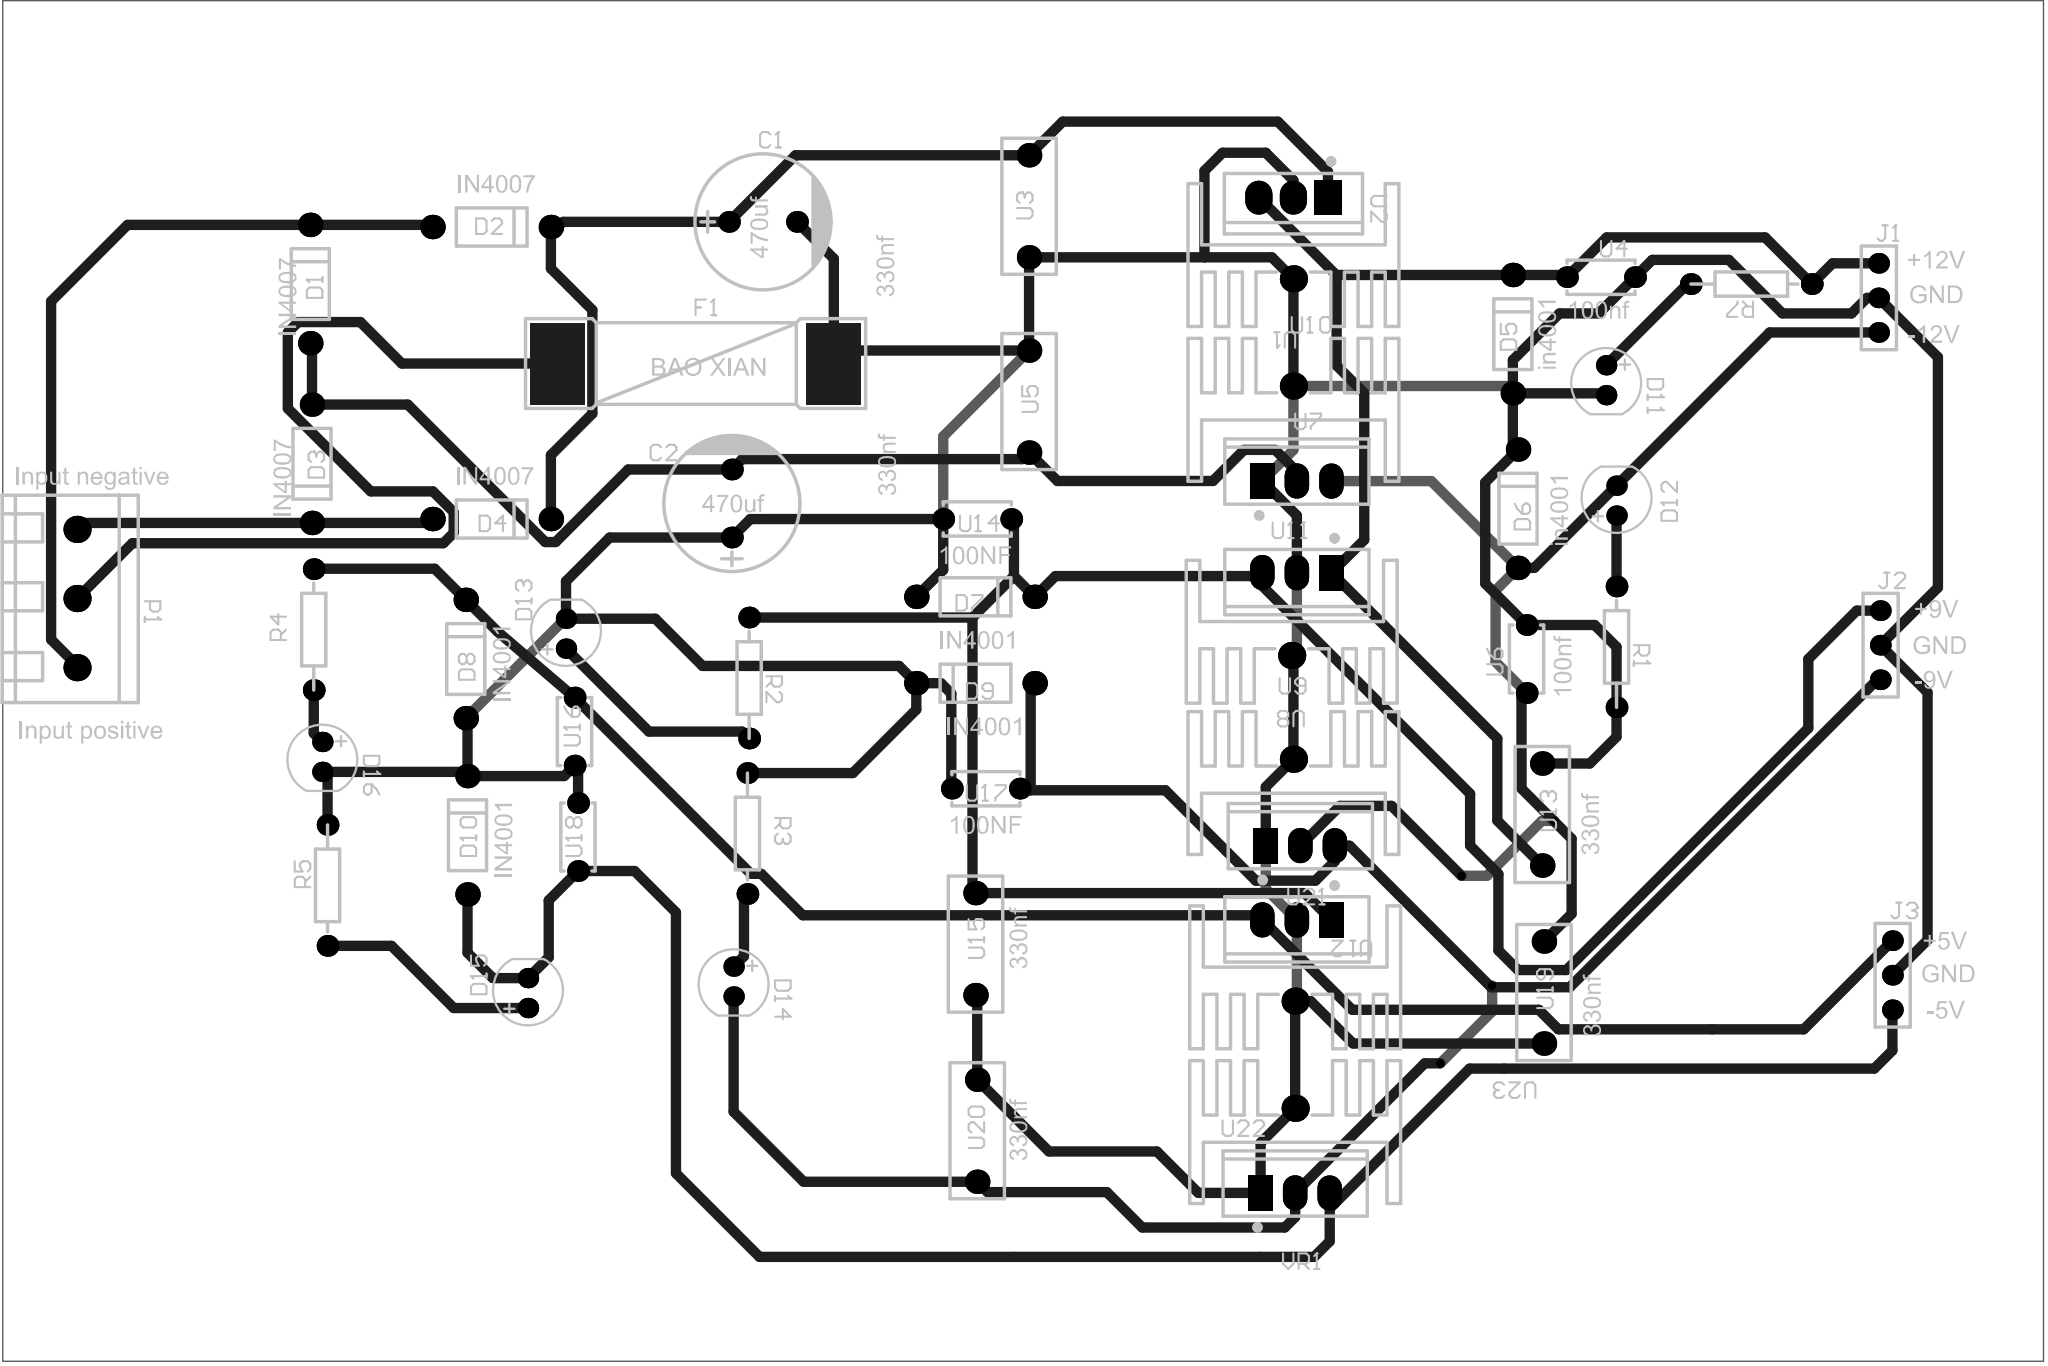Circuit board layout | Altium Designer
Layer stack:
# Altium Designer layer stack of  (unit mm; dielectric type: 0 none, 1 core, 2 prepreg, 3 surface material)
index,name,kind,layer,copper_thickness_mm,dielectric_type,dielectric_thickness_mm,dielectric_material,dielectric_constant
0,Top Silkscreen Layer,other,,,,,,
1,Top Paste Mask Layer,other,,,,,,
2,Top Solder Mask Layer,dielectric,,,3,0,,0
3,Top Layer,copper,Top Layer,0,,,,
4,Substrate-1,dielectric,,,3,0,,0
5,Bottom Layer,copper,Bottom Layer,0,,,,
6,Bottom Solder Mask Layer,dielectric,,,3,0,,0
7,Bottom Paste Mask Layer,other,,,,,,
8,Bottom Silkscreen Layer,other,,,,,,
# drill layer pairs: low layer,high layer
drill_pair,Top Layer,Bottom Layer
Part placement:
Designator,Comment,Layer,Footprint,Center-X(mm),Center-Y(mm),Rotation
D16,Red,TopLayer,发光二极管,99.794,120.617,270
D15,Red,TopLayer,发光二极管,114.907,103.259,90
D14,Red,TopLayer,发光二极管,130.02,104.107,270
D13,Red,TopLayer,发光二极管,117.701,129.675,90
D12,Red,TopLayer,发光二极管,194.917,139.454,90
D11,Red,TopLayer,发光二极管,194.155,148.303,270
VR1,L7905,TopLayer,TO-220-3_L10.0-W4.5-P2.54-L,171.295,88.57,0
U21,LM7909CT,TopLayer,TO-220-3_L10.0-W4.5-P2.54-L,171.676,114.097,0
U12,L7805CV-DG,TopLayer,TO-220-3_L10.0-W4.5-P2.54-L,171.422,108.636,180
U11,L7809CV,TopLayer,TO-220-3_L10.0-W4.5-P2.54-L,171.422,134.163,180
U7,L7912CV,TopLayer,TO-220-3_L10.0-W4.5-P2.54-L,171.422,140.894,0
U18,100NF,TopLayer,CAP-TH_L5.0-W2.5-P5.00-D1.0,118.59,114.732,270
U17,100NF,TopLayer,CAP-TH_L5.0-W2.5-P5.00-D1.0,148.562,118.288,0
U16,100NF,TopLayer,CAP-TH_L5.0-W2.5-P5.00-D1.0,118.336,122.479,270
U14,100NF,TopLayer,CAP-TH_L5.0-W2.5-P5.00-D1.0,147.927,138.1,180
U6,100NF,TopLayer,CAP-TH_L5.0-W2.5-P5.00-D1.0,188.313,127.813,270
U4,100NF,TopLayer,CAP-TH_L5.0-W2.5-P5.00-D1.0,193.774,155.88,0
U20,330nF,TopLayer,CAP-TH_L10.0-W4.0-P7.50-D0.6-1,147.927,93.142,90
U19,330nF,TopLayer,CAP-TH_L10.0-W4.0-P7.50-D0.6-1,189.583,103.302,270
U15,330nF,TopLayer,CAP-TH_L10.0-W4.0-P7.50-D0.6-1,147.8,106.858,90
U13,330nF,TopLayer,CAP-TH_L10.0-W4.0-P7.50-D0.6-1,189.456,116.383,270
U5,330nF,TopLayer,CAP-TH_L10.0-W4.0-P7.50-D0.6-1,151.737,146.736,90
U3,330nF,TopLayer,CAP-TH_L10.0-W4.0-P7.50-D0.6-1,151.737,161.087,90
U2,L7812CV,TopLayer,TO-220-3_L10.0-W4.5-P2.54-T,171.168,161.722,270
U23,15*10.5*21,TopLayer,SINK-TH_L15.0-W10.5-H21.0,171.295,102.667,180
U22,15*10.5*21,TopLayer,SINK-TH_L15.0-W10.5-H21.0,171.295,94.793,0
U10,15*10.5*21,TopLayer,SINK-TH_L15.0-W10.5-H21.0,171.168,147.879,0
U9,15*10.5*21,TopLayer,SINK-TH_L15.0-W10.5-H21.0,171.168,120.447,0
U8,15*10.5*21,TopLayer,SINK-TH_L15.0-W10.5-H21.0,171.041,128.067,180
U1,15*10.5*21,TopLayer,SINK-TH_L15.0-W10.5-H21.0,171.168,155.753,180
R7,10k 1/4W,TopLayer,10KÖ±²åµç×è_PCB·â×°,204.823,155.372,180
R5,10k 1/4W,TopLayer,10KÖ±²åµç×è_PCB·â×°,100.175,111.176,90
R4,10k 1/4W,TopLayer,10KÖ±²åµç×è_PCB·â×°,99.159,129.972,270
R3,10k 1/4W,TopLayer,10KÖ±²åµç×è_PCB·â×°,131.036,114.986,90
R2,10k 1/4W,TopLayer,10KÖ±²åµç×è_PCB·â×°,131.163,126.416,270
R1,10k 1/4W,TopLayer,10KÖ±²åµç×è_PCB·â×°,194.917,128.702,270
P1,WJ500V-5.08-3P,TopLayer,CONN-TH_3P-P5.00_WJ500V-5.08-3P,81.76,132.258,270
J3,1*3 pin header,TopLayer,1*3排针,215.194,104.572,0
J2,1*3 pin header,TopLayer,1*3排针,214.305,128.829,0
J1,1*3 pin header,TopLayer,1*3排针,214.178,154.356,0
F1,10A,TopLayer,FUSE-SMD_5-20MM,127.226,149.53,0
D10,IN4001,TopLayer,DO-41_BD2.4-L4.7-P8.70-D0.9-RD,110.462,114.859,270
D9,IN4001,TopLayer,DO-41_BD2.4-L4.7-P8.70-D0.9-RD,147.8,126.035,0
D8,IN4001,TopLayer,DO-41_BD2.4-L4.7-P8.70-D0.9-RD,110.335,127.813,270
D7,IN4001,TopLayer,DO-41_BD2.4-L4.7-P8.70-D0.9-RD,147.8,132.385,180
D6,IN4001,TopLayer,DO-41_BD2.4-L4.7-P8.70-D0.9-RD,187.678,138.862,270
D5,IN4001,TopLayer,DO-41_BD2.4-L4.7-P8.70-D0.9-RD,187.297,151.689,270
D4,1N4007,TopLayer,DO-41_BD2.4-L4.7-P8.70-D0.9-RD,112.24,138.1,180
D3,1N4007,TopLayer,DO-41_BD2.4-L4.7-P8.70-D0.9-RD,99.032,142.164,90
D2,1N4007,TopLayer,DO-41_BD2.4-L4.7-P8.70-D0.9-RD,112.24,159.563,180
D1,1N4007,TopLayer,DO-41_BD2.4-L4.7-P8.70-D0.9-RD,98.905,155.372,270
C2,470uF,TopLayer,CAP-TH_BD10.0-P5.00-D0.6-FD,129.893,139.243,90
C1,470uF,TopLayer,CAP-TH_BD10.0-P5.00-D0.6-FD,132.179,159.944,0
Pad and via stacks:
# Altium Designer via and pad stacks of  (unit mm). Each distinct definition once, with the count of objects using it.
# via: kind,start_layer,end_layer,hole_mm,diameter_mm,mode(0 simple;1 top-mid-bottom;2 full stack),diameter_per_layer,count,example_net
# pad: kind,layer,hole_mm,hole_type(0 round;1 square;2 slot),plating,top_size,top_shape(1 round;2 rect;3 octagon;9 rounded rect),mid_size,bottom_size,mode,footprint,size_per_layer,count,example
pad,Multi-Layer,0.8001,2,plated,1.5x1.5,1,1.5x1.5,1.5x1.5,0,\u00B7\u00A2\u00B9\u00E2\u00B6\u00FE\u00BC\u00AB\u00B9\u00DC,,12,D16.1
pad,Multi-Layer,1.2,2,plated,1.8x2.6,1,1.8x2.6,1.8x2.6,0,TO-220-3_L10.0-W4.5-P2.54-L,,2,VR1.2
pad,Multi-Layer,1.2,2,plated,1.8x2.6,2,1.8x2.6,1.8x2.6,0,TO-220-3_L10.0-W4.5-P2.54-L,,1,VR1.1
pad,Multi-Layer,1.2,0,plated,1.8x2.6,1,1.8x2.6,1.8x2.6,0,TO-220-3_L10.0-W4.5-P2.54-L,,8,U21.2
pad,Multi-Layer,1.2,0,plated,1.8x2.6,2,1.8x2.6,1.8x2.6,0,TO-220-3_L10.0-W4.5-P2.54-L,,4,U21.1
pad,Multi-Layer,1,0,plated,1.6x1.6,1,1.6x1.6,1.6x1.6,0,CAP-TH_L5.0-W2.5-P5.00-D1.0,,12,U18.1
pad,Multi-Layer,1,0,plated,1.8x1.8,1,1.8x1.8,1.8x1.8,0,CAP-TH_L10.0-W4.0-P7.50-D0.6-1,,12,U20.2
pad,Multi-Layer,1.3,0,plated,2x2.5,2,2x2.5,2x2.5,0,TO-220-3_L10.0-W4.5-P2.54-T,,1,U2.1
pad,Multi-Layer,1.3,0,plated,2x2.5,1,2x2.5,2x2.5,0,TO-220-3_L10.0-W4.5-P2.54-T,,2,U2.3
pad,Multi-Layer,1.5,0,plated,2x2,1,2x2,2x2,0,SINK-TH_L15.0-W10.5-H21.0,,6,U23.1
pad,Multi-Layer,0.92,2,plated,1.6x1.6,1,1.6x1.6,1.6x1.6,0,10K\u00D6\u00B1\u00B2\u00E5\u00B5\u00E7\u00D7\u00E8 PCB\u00B7\u00E2\u00D7\u00B0,,12,R7.1
pad,Multi-Layer,1.3,0,plated,2x2,1,2x2,2x2,0,CONN-TH_3P-P5.00_WJ500V-5.08-3P,,3,P1.3
pad,Multi-Layer,0.9144,0,plated,1.524x1.524,1,1.524x1.524,1.524x1.524,0,1*3\u00C5\u00C5\u00D5\u00EB,,9,J3.3
pad,Multi-Layer,1,0,plated,1.8x1.8,1,1.8x1.8,1.8x1.8,0,DO-41_BD2.4-L4.7-P8.70-D0.9-RD,,20,D10.1
pad,Multi-Layer,1,0,plated,1.6x1.6,1,1.6x1.6,1.6x1.6,0,CAP-TH_BD10.0-P5.00-D0.6-FD,,4,C2.2
pad,Top Layer,0,0,plated,4x6,2,4x6,4x6,0,FUSE-SMD_5-20MM,,2,F1.1
via,Top Layer,Bottom Layer,0.3048,0.61,0,,4,U7_3
Design rules, without the lines most boards share:
# Altium Designer design rules of  (exported by Altium Designer, unit mm)
# columns: name | kind | enabled | priority | scope1 | scope2 | descriptor | typed fields (field=value)
Plane_Default | 0 | disabled | 1 | All | All | Clearance Constraint (Gap=6mil) (Disabled)(All),(All) | gap=0.1524
Plane_Default_1 | 63 | disabled | 1 | All | All | Board Clearance Constraint (Gap=0mil) (Disabled)(All) |
Copper_Default | 0 | disabled | 2 | All | All | Clearance Constraint (Gap=6mil) (Disabled)(All),(All) | gap=0.1524
Copper_Default_1 | 63 | disabled | 2 | All | All | Board Clearance Constraint (Gap=0mil) (Disabled)(All) |
Copper_gge8332 | 0 | disabled | 3 | All | All | Clearance Constraint (Gap=6mil) (Disabled)(All),(All) | gap=0.1524
Copper_gge8332_1 | 63 | disabled | 3 | All | All | Board Clearance Constraint (Gap=0mil) (Disabled)(All) |
Copper_gge8326 | 0 | disabled | 4 | All | All | Clearance Constraint (Gap=6mil) (Disabled)(All),(All) | gap=0.1524
Copper_gge8326_1 | 63 | disabled | 4 | All | All | Board Clearance Constraint (Gap=0mil) (Disabled)(All) |
Default | 0 | enabled | 5 | All | All | Clearance Constraint (Gap=6mil) (All),(All) | gap=0.1524
Default_1 | 63 | enabled | 5 | All | All | Board Clearance Constraint (Gap=0mil) (All) |
Default_2 | 2 | enabled | 1 | All | All | Width Constraint (Min=30mil) (Max=1000mil) (Preferred=30mil) (All) |
Default_3 | 11 | enabled | 1 | All | All | Routing Via (MinHoleWidth=12mil) (MaxHoleWidth=2362mil) (PreferredHoleWidth=12mil) (MinWidth=24mil) (MaxWidth=3938mil) (PreferedWidth=24mil) (All) | via_min_hole=0.3048 via_max_hole=59.995 via_preferred_diameter=0.6096 via_preferred_hole=0.3048
Default_4 | 6 | enabled | 1 | All | All | Power Plane Connect Rule(Relief Connect )(Expansion=20mil) (Conductor Width=0mil) (Air Gap=10mil) (Entries=4) (All) | relief_conductor_width=0 relief_entries=4 relief_expansion=0.508
gge8332 | 20 | disabled | 1 | All | All | Polygon Connect Rule(Relief Connect )(Conductor Width=0mil) (Relief Angle=90 Angle) (Entries=4) (Air Gap Width=1mil) (Disabled)(All),(All) | connect_style(0=relief,1=direct,2=none)=0 relief_conductor_width=0 relief_entries=4
gge8326 | 20 | disabled | 2 | All | All | Polygon Connect Rule(Relief Connect )(Conductor Width=0mil) (Relief Angle=90 Angle) (Entries=4) (Air Gap Width=1mil) (Disabled)(All),(All) | connect_style(0=relief,1=direct,2=none)=0 relief_conductor_width=0 relief_entries=4
Default_5 | 20 | enabled | 3 | All | All | Polygon Connect Rule(Relief Connect )(Conductor Width=0mil) (Relief Angle=90 Angle) (Entries=4) (Air Gap Width=1mil) (All),(All) | connect_style(0=relief,1=direct,2=none)=0 relief_conductor_width=0 relief_entries=4
Common | 14 | enabled | 1 | All | All | Paste Mask Expansion (Expansion =0mil) (All) | expansion=0
Common_1 | 13 | enabled | 2 | All | All | Solder Mask Expansion (Expansion =2mil) (All) | expansion=0.0508
Common_2 | 13 | enabled | 1 | IsVia | All | Solder Mask Expansion (Expansion =-1000mil) (IsVia) | expansion=-25.4